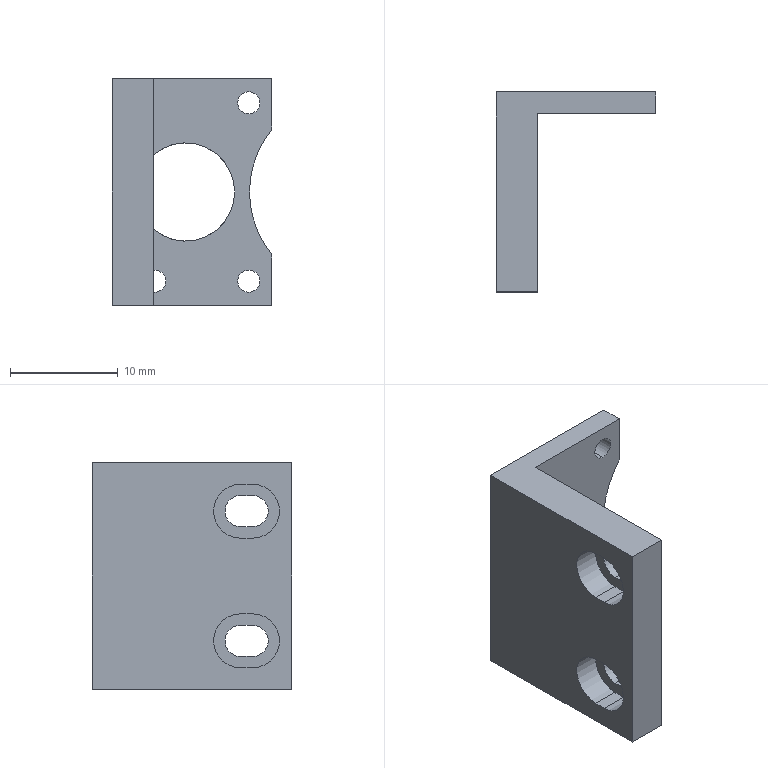Part | STEP file | 1 solid | 39 faces | box 14.8 x 18.5 x 21 mm | volume 1569 mm3 | plane 20 | cylinder 18 | cone 1 | commonest cylinder face diameters 2.05 x6 2.9 x4 5 x4 9.1 x2 18.5 x2